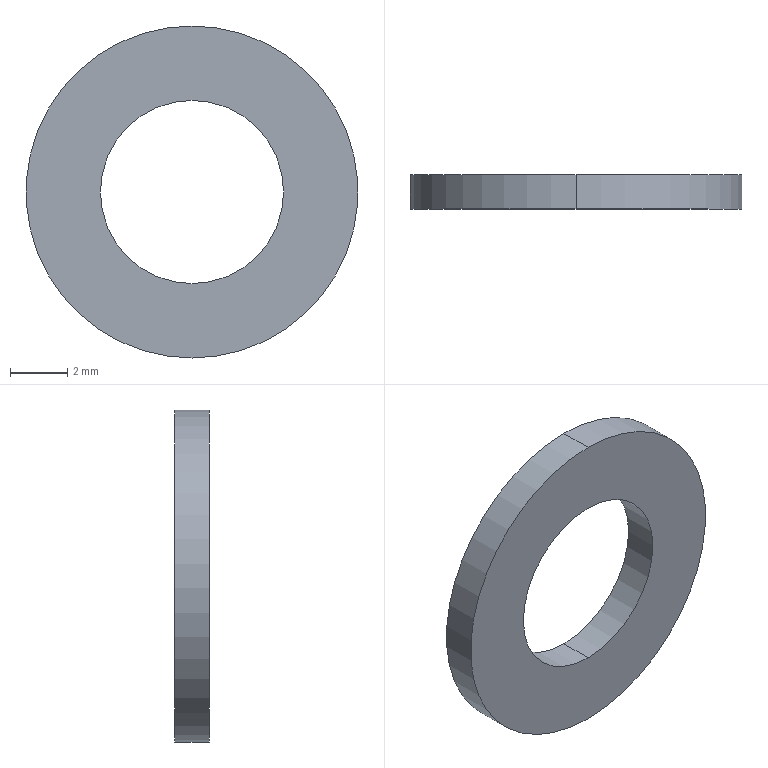Part | SolidWorks | features Extrusion 1 | 1 solid | 6 faces | box 11.6 x 1.2 x 11.6 mm | volume 88.216 mm3 | cylinder 4 | plane 2 | commonest cylinder face diameters 6.4 x2 11.6 x2
STEP:
#1=CARTESIAN_POINT('',(0.,1.2,-3.2));
#2=VERTEX_POINT('',#1);
#3=CARTESIAN_POINT('',(0.,1.2,3.2));
#4=VERTEX_POINT('',#3);
#5=CARTESIAN_POINT('',(0.,1.2,0.));
#6=DIRECTION('',(0.,1.,0.));
#7=DIRECTION('',(0.,0.,1.));
#8=AXIS2_PLACEMENT_3D('',#5,#6,#7);
#9=CIRCLE('',#8,3.2);
#10=EDGE_CURVE('',#2,#4,#9,.T.);
#11=ORIENTED_EDGE('',*,*,#10,.T.);
#12=CARTESIAN_POINT('',(0.,0.,3.2));
#13=VERTEX_POINT('',#12);
#14=CARTESIAN_POINT('',(0.,1.2,3.2));
#15=DIRECTION('',(0.,-1.,0.));
#16=VECTOR('',#15,1000.);
#17=LINE('',#14,#16);
#18=EDGE_CURVE('',#4,#13,#17,.T.);
#19=ORIENTED_EDGE('',*,*,#18,.T.);
#20=CARTESIAN_POINT('',(0.,0.,-3.2));
#21=VERTEX_POINT('',#20);
#22=CARTESIAN_POINT('',(0.,0.,0.));
#23=DIRECTION('',(0.,1.,0.));
#24=DIRECTION('',(0.,0.,1.));
#25=AXIS2_PLACEMENT_3D('',#22,#23,#24);
#26=CIRCLE('',#25,3.2);
#27=EDGE_CURVE('',#21,#13,#26,.T.);
#28=ORIENTED_EDGE('',*,*,#27,.F.);
#29=CARTESIAN_POINT('',(0.,1.2,-3.2));
#30=DIRECTION('',(0.,-1.,0.));
#31=VECTOR('',#30,1000.);
#32=LINE('',#29,#31);
#33=EDGE_CURVE('',#2,#21,#32,.T.);
#34=ORIENTED_EDGE('',*,*,#33,.F.);
#35=EDGE_LOOP('',(#11,#19,#28,#34));
#36=FACE_OUTER_BOUND('',#35,.T.);
#37=CARTESIAN_POINT('',(0.,1.2,0.));
#38=DIRECTION('',(0.,-1.,0.));
#39=DIRECTION('',(0.,0.,-1.));
#40=AXIS2_PLACEMENT_3D('',#37,#38,#39);
#41=CYLINDRICAL_SURFACE('',#40,3.2);
#42=ADVANCED_FACE('',(#36),#41,.F.);
#43=CARTESIAN_POINT('',(0.,1.2,5.8));
#44=VERTEX_POINT('',#43);
#45=CARTESIAN_POINT('',(0.,1.2,-5.8));
#46=VERTEX_POINT('',#45);
#47=CARTESIAN_POINT('',(0.,1.2,0.));
#48=DIRECTION('',(0.,1.,0.));
#49=DIRECTION('',(0.,0.,1.));
#50=AXIS2_PLACEMENT_3D('',#47,#48,#49);
#51=CIRCLE('',#50,5.8);
#52=EDGE_CURVE('',#44,#46,#51,.T.);
#53=ORIENTED_EDGE('',*,*,#52,.F.);
#54=CARTESIAN_POINT('',(0.,0.,5.8));
#55=VERTEX_POINT('',#54);
#56=CARTESIAN_POINT('',(0.,1.2,5.8));
#57=DIRECTION('',(0.,-1.,0.));
#58=VECTOR('',#57,1000.);
#59=LINE('',#56,#58);
#60=EDGE_CURVE('',#44,#55,#59,.T.);
#61=ORIENTED_EDGE('',*,*,#60,.T.);
#62=CARTESIAN_POINT('',(0.,0.,-5.8));
#63=VERTEX_POINT('',#62);
#64=CARTESIAN_POINT('',(0.,0.,0.));
#65=DIRECTION('',(0.,1.,0.));
#66=DIRECTION('',(0.,0.,1.));
#67=AXIS2_PLACEMENT_3D('',#64,#65,#66);
#68=CIRCLE('',#67,5.8);
#69=EDGE_CURVE('',#55,#63,#68,.T.);
#70=ORIENTED_EDGE('',*,*,#69,.T.);
#71=CARTESIAN_POINT('',(0.,1.2,-5.8));
#72=DIRECTION('',(0.,-1.,0.));
#73=VECTOR('',#72,1000.);
#74=LINE('',#71,#73);
#75=EDGE_CURVE('',#46,#63,#74,.T.);
#76=ORIENTED_EDGE('',*,*,#75,.F.);
#77=EDGE_LOOP('',(#53,#61,#70,#76));
#78=FACE_OUTER_BOUND('',#77,.T.);
#79=CARTESIAN_POINT('',(0.,1.2,0.));
#80=DIRECTION('',(0.,-1.,0.));
#81=DIRECTION('',(0.,0.,-1.));
#82=AXIS2_PLACEMENT_3D('',#79,#80,#81);
#83=CYLINDRICAL_SURFACE('',#82,5.8);
#84=ADVANCED_FACE('',(#78),#83,.T.);
#85=CARTESIAN_POINT('',(0.,1.2,0.));
#86=DIRECTION('',(0.,1.,0.));
#87=DIRECTION('',(0.,0.,1.));
#88=AXIS2_PLACEMENT_3D('',#85,#86,#87);
#89=CIRCLE('',#88,5.8);
#90=EDGE_CURVE('',#46,#44,#89,.T.);
#91=ORIENTED_EDGE('',*,*,#90,.T.);
#92=ORIENTED_EDGE('',*,*,#52,.T.);
#93=EDGE_LOOP('',(#91,#92));
#94=FACE_OUTER_BOUND('',#93,.T.);
#95=ORIENTED_EDGE('',*,*,#10,.F.);
#96=CARTESIAN_POINT('',(0.,1.2,0.));
#97=DIRECTION('',(0.,1.,0.));
#98=DIRECTION('',(0.,0.,1.));
#99=AXIS2_PLACEMENT_3D('',#96,#97,#98);
#100=CIRCLE('',#99,3.2);
#101=EDGE_CURVE('',#4,#2,#100,.T.);
#102=ORIENTED_EDGE('',*,*,#101,.F.);
#103=EDGE_LOOP('',(#95,#102));
#104=FACE_BOUND('',#103,.T.);
#105=CARTESIAN_POINT('',(0.,1.2,0.));
#106=DIRECTION('',(0.,1.,0.));
#107=DIRECTION('',(0.,0.,1.));
#108=AXIS2_PLACEMENT_3D('',#105,#106,#107);
#109=PLANE('',#108);
#110=ADVANCED_FACE('',(#94,#104),#109,.T.);
#111=CARTESIAN_POINT('',(0.,0.,0.));
#112=DIRECTION('',(0.,1.,0.));
#113=DIRECTION('',(0.,0.,1.));
#114=AXIS2_PLACEMENT_3D('',#111,#112,#113);
#115=CIRCLE('',#114,5.8);
#116=EDGE_CURVE('',#63,#55,#115,.T.);
#117=ORIENTED_EDGE('',*,*,#116,.F.);
#118=ORIENTED_EDGE('',*,*,#69,.F.);
#119=EDGE_LOOP('',(#117,#118));
#120=FACE_OUTER_BOUND('',#119,.T.);
#121=ORIENTED_EDGE('',*,*,#27,.T.);
#122=CARTESIAN_POINT('',(0.,0.,0.));
#123=DIRECTION('',(0.,1.,0.));
#124=DIRECTION('',(0.,0.,1.));
#125=AXIS2_PLACEMENT_3D('',#122,#123,#124);
#126=CIRCLE('',#125,3.2);
#127=EDGE_CURVE('',#13,#21,#126,.T.);
#128=ORIENTED_EDGE('',*,*,#127,.T.);
#129=EDGE_LOOP('',(#121,#128));
#130=FACE_BOUND('',#129,.T.);
#131=CARTESIAN_POINT('',(0.,0.,0.));
#132=DIRECTION('',(0.,1.,0.));
#133=DIRECTION('',(0.,0.,1.));
#134=AXIS2_PLACEMENT_3D('',#131,#132,#133);
#135=PLANE('',#134);
#136=ADVANCED_FACE('',(#120,#130),#135,.F.);
#137=ORIENTED_EDGE('',*,*,#60,.F.);
#138=ORIENTED_EDGE('',*,*,#90,.F.);
#139=ORIENTED_EDGE('',*,*,#75,.T.);
#140=ORIENTED_EDGE('',*,*,#116,.T.);
#141=EDGE_LOOP('',(#137,#138,#139,#140));
#142=FACE_OUTER_BOUND('',#141,.T.);
#143=CARTESIAN_POINT('',(0.,1.2,0.));
#144=DIRECTION('',(0.,-1.,0.));
#145=DIRECTION('',(0.,0.,-1.));
#146=AXIS2_PLACEMENT_3D('',#143,#144,#145);
#147=CYLINDRICAL_SURFACE('',#146,5.8);
#148=ADVANCED_FACE('',(#142),#147,.T.);
#149=ORIENTED_EDGE('',*,*,#18,.F.);
#150=ORIENTED_EDGE('',*,*,#101,.T.);
#151=ORIENTED_EDGE('',*,*,#33,.T.);
#152=ORIENTED_EDGE('',*,*,#127,.F.);
#153=EDGE_LOOP('',(#149,#150,#151,#152));
#154=FACE_OUTER_BOUND('',#153,.T.);
#155=CARTESIAN_POINT('',(0.,1.2,0.));
#156=DIRECTION('',(0.,-1.,0.));
#157=DIRECTION('',(0.,0.,-1.));
#158=AXIS2_PLACEMENT_3D('',#155,#156,#157);
#159=CYLINDRICAL_SURFACE('',#158,3.2);
#160=ADVANCED_FACE('',(#154),#159,.F.);
#161=CLOSED_SHELL('',(#42,#84,#110,#136,#148,#160));
#162=MANIFOLD_SOLID_BREP('',#161);
#163=CARTESIAN_POINT('',(0.,0.,0.));
#164=DIRECTION('',(0.,0.,1.));
#165=DIRECTION('',(1.,0.,0.));
#166=AXIS2_PLACEMENT_3D('',#163,#164,#165);
#167=(LENGTH_UNIT()NAMED_UNIT(*)SI_UNIT(.MILLI.,.METRE.));
#168=UNCERTAINTY_MEASURE_WITH_UNIT(LENGTH_MEASURE(0.00001),#167,'','');
#169=(NAMED_UNIT(*)PLANE_ANGLE_UNIT()SI_UNIT($,.RADIAN.));
#170=(NAMED_UNIT(*)SI_UNIT($,.STERADIAN.)SOLID_ANGLE_UNIT());
#171=(GEOMETRIC_REPRESENTATION_CONTEXT(3)GLOBAL_UNCERTAINTY_ASSIGNED_CONTEXT((#168))GLOBAL_UNIT_ASSIGNED_CONTEXT((#167,#169,#170))REPRESENTATION_CONTEXT('',''));
#172=ADVANCED_BREP_SHAPE_REPRESENTATION('',(#162,#166),#171);